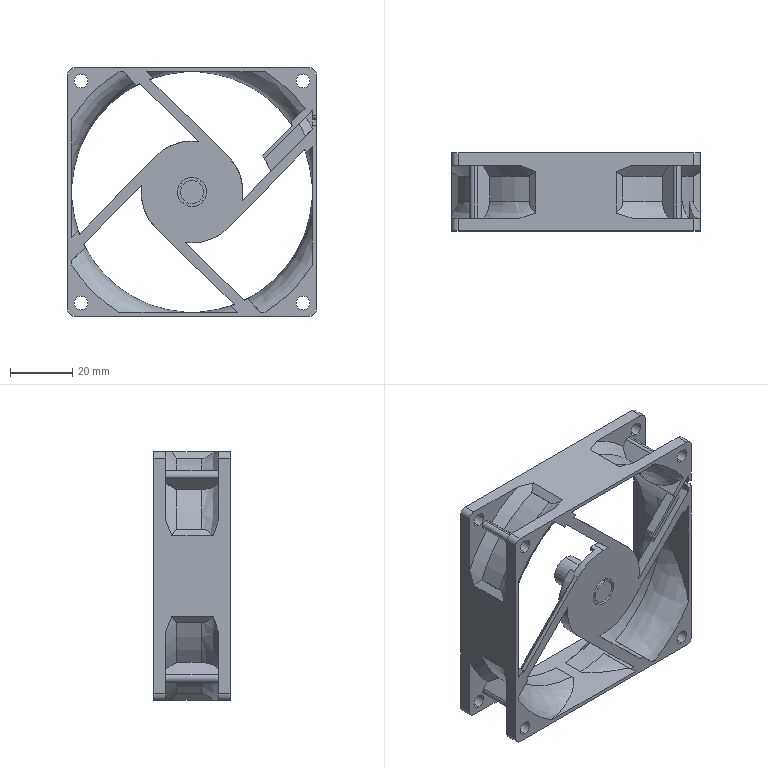Part | STEP file | 8025R_9_1 | 1 solid | 237 faces | box 80 x 25 x 80 mm | volume 22604 mm3 | plane 120 | cylinder 88 | spline 17 | cone 12 | commonest cylinder face diameters 4 x24 4.4 x16 81.5 x8 2.8 x6 7.4 x5 9.4 x5